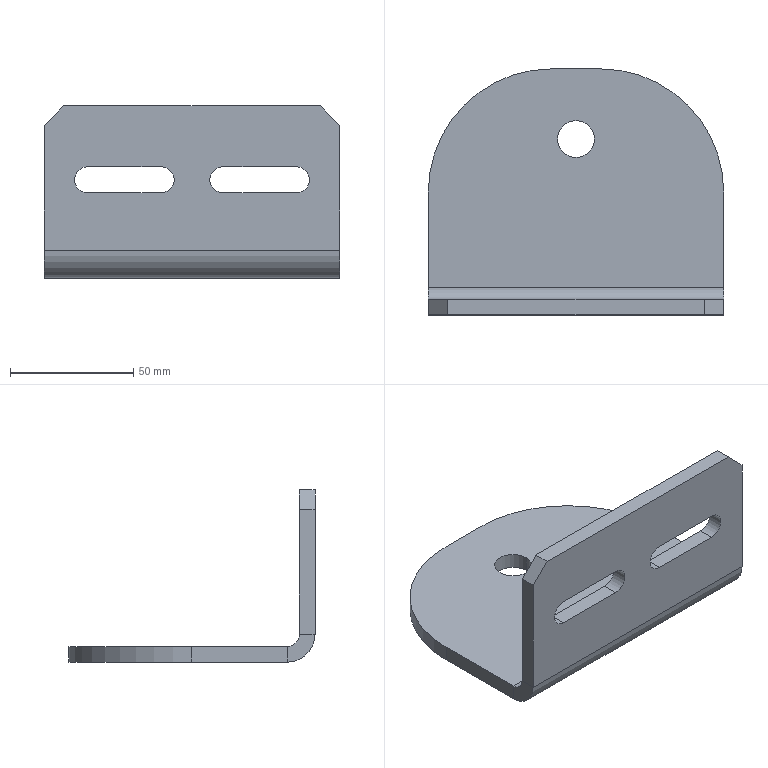Part | STEP file | BASE POLEA_B_SHEET METAL | 1 solid | 28 faces | box 120 x 100 x 70 mm | volume 108585 mm3 | plane 18 | cylinder 10 | commonest cylinder face diameters 10.5 x4 15 x2 100 x2 10 x1 22.7 x1
STEP:
#1=CARTESIAN_POINT('',(-7.5,71.5,0.));
#2=VERTEX_POINT('',#1);
#3=CARTESIAN_POINT('',(7.5,71.5,0.));
#4=VERTEX_POINT('',#3);
#5=CARTESIAN_POINT('',(0.,71.5,0.));
#6=DIRECTION('',(0.,0.,1.));
#7=DIRECTION('',(1.,0.,0.));
#8=AXIS2_PLACEMENT_3D('',#5,#6,#7);
#9=CIRCLE('',#8,7.5);
#10=EDGE_CURVE('',#2,#4,#9,.T.);
#11=ORIENTED_EDGE('',*,*,#10,.F.);
#12=CARTESIAN_POINT('',(-7.5,71.5,6.35));
#13=VERTEX_POINT('',#12);
#14=CARTESIAN_POINT('',(-7.5,71.5,-3.65));
#15=DIRECTION('',(0.,0.,1.));
#16=VECTOR('',#15,1000.);
#17=LINE('',#14,#16);
#18=EDGE_CURVE('',#2,#13,#17,.T.);
#19=ORIENTED_EDGE('',*,*,#18,.T.);
#20=CARTESIAN_POINT('',(7.5,71.5,6.35));
#21=VERTEX_POINT('',#20);
#22=CARTESIAN_POINT('',(0.,71.5,6.35));
#23=DIRECTION('',(0.,0.,1.));
#24=DIRECTION('',(1.,0.,0.));
#25=AXIS2_PLACEMENT_3D('',#22,#23,#24);
#26=CIRCLE('',#25,7.5);
#27=EDGE_CURVE('',#13,#21,#26,.T.);
#28=ORIENTED_EDGE('',*,*,#27,.T.);
#29=CARTESIAN_POINT('',(7.5,71.5,-3.65));
#30=DIRECTION('',(0.,0.,1.));
#31=VECTOR('',#30,1000.);
#32=LINE('',#29,#31);
#33=EDGE_CURVE('',#4,#21,#32,.T.);
#34=ORIENTED_EDGE('',*,*,#33,.F.);
#35=EDGE_LOOP('',(#11,#19,#28,#34));
#36=FACE_OUTER_BOUND('',#35,.T.);
#37=CARTESIAN_POINT('',(0.,71.5,-3.65));
#38=DIRECTION('',(0.,0.,1.));
#39=DIRECTION('',(1.,0.,0.));
#40=AXIS2_PLACEMENT_3D('',#37,#38,#39);
#41=CYLINDRICAL_SURFACE('',#40,7.5);
#42=ADVANCED_FACE('',(#36),#41,.F.);
#43=CARTESIAN_POINT('',(60.,0.,11.35));
#44=VERTEX_POINT('',#43);
#45=CARTESIAN_POINT('',(60.,6.35,11.35));
#46=VERTEX_POINT('',#45);
#47=CARTESIAN_POINT('',(60.,0.,11.35));
#48=DIRECTION('',(0.,1.,0.));
#49=VECTOR('',#48,1000.);
#50=LINE('',#47,#49);
#51=EDGE_CURVE('',#44,#46,#50,.T.);
#52=ORIENTED_EDGE('',*,*,#51,.F.);
#53=CARTESIAN_POINT('',(60.,11.35,0.));
#54=VERTEX_POINT('',#53);
#55=CARTESIAN_POINT('',(60.,11.35,11.35));
#56=DIRECTION('',(1.,0.,0.));
#57=DIRECTION('',(0.,0.,1.));
#58=AXIS2_PLACEMENT_3D('',#55,#56,#57);
#59=CIRCLE('',#58,11.35);
#60=EDGE_CURVE('',#44,#54,#59,.T.);
#61=ORIENTED_EDGE('',*,*,#60,.T.);
#62=CARTESIAN_POINT('',(60.,11.35,6.35));
#63=VERTEX_POINT('',#62);
#64=CARTESIAN_POINT('',(60.,11.35,6.35));
#65=DIRECTION('',(0.,0.,-1.));
#66=VECTOR('',#65,1000.);
#67=LINE('',#64,#66);
#68=EDGE_CURVE('',#63,#54,#67,.T.);
#69=ORIENTED_EDGE('',*,*,#68,.F.);
#70=CARTESIAN_POINT('',(60.,11.35,11.35));
#71=DIRECTION('',(1.,0.,0.));
#72=DIRECTION('',(0.,0.,-1.));
#73=AXIS2_PLACEMENT_3D('',#70,#71,#72);
#74=CIRCLE('',#73,5.);
#75=EDGE_CURVE('',#46,#63,#74,.T.);
#76=ORIENTED_EDGE('',*,*,#75,.F.);
#77=EDGE_LOOP('',(#52,#61,#69,#76));
#78=FACE_OUTER_BOUND('',#77,.T.);
#79=CARTESIAN_POINT('',(60.,0.,11.35));
#80=DIRECTION('',(1.,0.,0.));
#81=DIRECTION('',(0.,0.,-1.));
#82=AXIS2_PLACEMENT_3D('',#79,#80,#81);
#83=PLANE('',#82);
#84=ADVANCED_FACE('',(#78),#83,.T.);
#85=CARTESIAN_POINT('',(60.,6.35,62.));
#86=VERTEX_POINT('',#85);
#87=CARTESIAN_POINT('',(60.,6.35,70.));
#88=DIRECTION('',(0.,0.,-1.));
#89=VECTOR('',#88,1000.);
#90=LINE('',#87,#89);
#91=EDGE_CURVE('',#86,#46,#90,.T.);
#92=ORIENTED_EDGE('',*,*,#91,.F.);
#93=CARTESIAN_POINT('',(60.,0.,62.));
#94=VERTEX_POINT('',#93);
#95=CARTESIAN_POINT('',(60.,11.35,62.));
#96=DIRECTION('',(0.,-1.,0.));
#97=VECTOR('',#96,1000.);
#98=LINE('',#95,#97);
#99=EDGE_CURVE('',#86,#94,#98,.T.);
#100=ORIENTED_EDGE('',*,*,#99,.T.);
#101=CARTESIAN_POINT('',(60.,0.,70.));
#102=DIRECTION('',(0.,0.,-1.));
#103=VECTOR('',#102,1000.);
#104=LINE('',#101,#103);
#105=EDGE_CURVE('',#94,#44,#104,.T.);
#106=ORIENTED_EDGE('',*,*,#105,.T.);
#107=ORIENTED_EDGE('',*,*,#51,.T.);
#108=EDGE_LOOP('',(#92,#100,#106,#107));
#109=FACE_OUTER_BOUND('',#108,.T.);
#110=CARTESIAN_POINT('',(60.,11.35,6.35));
#111=DIRECTION('',(1.,0.,0.));
#112=DIRECTION('',(0.,0.,-1.));
#113=AXIS2_PLACEMENT_3D('',#110,#111,#112);
#114=PLANE('',#113);
#115=ADVANCED_FACE('',(#109),#114,.T.);
#116=CARTESIAN_POINT('',(-60.,11.35,0.));
#117=VERTEX_POINT('',#116);
#118=CARTESIAN_POINT('',(-60.,11.35,6.35));
#119=VERTEX_POINT('',#118);
#120=CARTESIAN_POINT('',(-60.,11.35,0.));
#121=DIRECTION('',(0.,0.,1.));
#122=VECTOR('',#121,1000.);
#123=LINE('',#120,#122);
#124=EDGE_CURVE('',#117,#119,#123,.T.);
#125=ORIENTED_EDGE('',*,*,#124,.F.);
#126=CARTESIAN_POINT('',(-60.,0.,11.35));
#127=VERTEX_POINT('',#126);
#128=CARTESIAN_POINT('',(-60.,11.35,11.35));
#129=DIRECTION('',(1.,0.,0.));
#130=DIRECTION('',(0.,0.,1.));
#131=AXIS2_PLACEMENT_3D('',#128,#129,#130);
#132=CIRCLE('',#131,11.35);
#133=EDGE_CURVE('',#127,#117,#132,.T.);
#134=ORIENTED_EDGE('',*,*,#133,.F.);
#135=CARTESIAN_POINT('',(-60.,6.35,11.35));
#136=VERTEX_POINT('',#135);
#137=CARTESIAN_POINT('',(-60.,6.35,11.35));
#138=DIRECTION('',(0.,-1.,0.));
#139=VECTOR('',#138,1000.);
#140=LINE('',#137,#139);
#141=EDGE_CURVE('',#136,#127,#140,.T.);
#142=ORIENTED_EDGE('',*,*,#141,.F.);
#143=CARTESIAN_POINT('',(-60.,11.35,11.35));
#144=DIRECTION('',(1.,0.,0.));
#145=DIRECTION('',(0.,0.,-1.));
#146=AXIS2_PLACEMENT_3D('',#143,#144,#145);
#147=CIRCLE('',#146,5.);
#148=EDGE_CURVE('',#136,#119,#147,.T.);
#149=ORIENTED_EDGE('',*,*,#148,.T.);
#150=EDGE_LOOP('',(#125,#134,#142,#149));
#151=FACE_OUTER_BOUND('',#150,.T.);
#152=CARTESIAN_POINT('',(-60.,11.35,0.));
#153=DIRECTION('',(-1.,0.,0.));
#154=DIRECTION('',(0.,0.,1.));
#155=AXIS2_PLACEMENT_3D('',#152,#153,#154);
#156=PLANE('',#155);
#157=ADVANCED_FACE('',(#151),#156,.T.);
#158=CARTESIAN_POINT('',(-60.,50.,6.35));
#159=VERTEX_POINT('',#158);
#160=CARTESIAN_POINT('',(-60.,0.,6.35));
#161=DIRECTION('',(0.,1.,0.));
#162=VECTOR('',#161,1000.);
#163=LINE('',#160,#162);
#164=EDGE_CURVE('',#119,#159,#163,.T.);
#165=ORIENTED_EDGE('',*,*,#164,.T.);
#166=CARTESIAN_POINT('',(-60.,50.,0.));
#167=VERTEX_POINT('',#166);
#168=CARTESIAN_POINT('',(-60.,50.,11.35));
#169=DIRECTION('',(0.,0.,-1.));
#170=VECTOR('',#169,1000.);
#171=LINE('',#168,#170);
#172=EDGE_CURVE('',#159,#167,#171,.T.);
#173=ORIENTED_EDGE('',*,*,#172,.T.);
#174=CARTESIAN_POINT('',(-60.,0.,0.));
#175=DIRECTION('',(0.,1.,0.));
#176=VECTOR('',#175,1000.);
#177=LINE('',#174,#176);
#178=EDGE_CURVE('',#117,#167,#177,.T.);
#179=ORIENTED_EDGE('',*,*,#178,.F.);
#180=ORIENTED_EDGE('',*,*,#124,.T.);
#181=EDGE_LOOP('',(#165,#173,#179,#180));
#182=FACE_OUTER_BOUND('',#181,.T.);
#183=CARTESIAN_POINT('',(-60.,6.35,11.35));
#184=DIRECTION('',(-1.,0.,0.));
#185=DIRECTION('',(0.,0.,1.));
#186=AXIS2_PLACEMENT_3D('',#183,#184,#185);
#187=PLANE('',#186);
#188=ADVANCED_FACE('',(#182),#187,.T.);
#189=CARTESIAN_POINT('',(0.,71.5,0.));
#190=DIRECTION('',(0.,0.,1.));
#191=DIRECTION('',(1.,0.,0.));
#192=AXIS2_PLACEMENT_3D('',#189,#190,#191);
#193=CIRCLE('',#192,7.5);
#194=EDGE_CURVE('',#4,#2,#193,.T.);
#195=ORIENTED_EDGE('',*,*,#194,.T.);
#196=ORIENTED_EDGE('',*,*,#10,.T.);
#197=EDGE_LOOP('',(#195,#196));
#198=FACE_BOUND('',#197,.T.);
#199=ORIENTED_EDGE('',*,*,#178,.T.);
#200=CARTESIAN_POINT('',(-10.,100.,0.));
#201=VERTEX_POINT('',#200);
#202=CARTESIAN_POINT('',(-10.,50.,0.));
#203=DIRECTION('',(0.,0.,-1.));
#204=DIRECTION('',(1.,0.,0.));
#205=AXIS2_PLACEMENT_3D('',#202,#203,#204);
#206=CIRCLE('',#205,50.);
#207=EDGE_CURVE('',#167,#201,#206,.T.);
#208=ORIENTED_EDGE('',*,*,#207,.T.);
#209=CARTESIAN_POINT('',(10.,100.,0.));
#210=VERTEX_POINT('',#209);
#211=CARTESIAN_POINT('',(60.,100.,0.));
#212=DIRECTION('',(-1.,0.,0.));
#213=VECTOR('',#212,1000.);
#214=LINE('',#211,#213);
#215=EDGE_CURVE('',#210,#201,#214,.T.);
#216=ORIENTED_EDGE('',*,*,#215,.F.);
#217=CARTESIAN_POINT('',(60.,50.,0.));
#218=VERTEX_POINT('',#217);
#219=CARTESIAN_POINT('',(10.,50.,0.));
#220=DIRECTION('',(0.,0.,-1.));
#221=DIRECTION('',(1.,0.,0.));
#222=AXIS2_PLACEMENT_3D('',#219,#220,#221);
#223=CIRCLE('',#222,50.);
#224=EDGE_CURVE('',#210,#218,#223,.T.);
#225=ORIENTED_EDGE('',*,*,#224,.T.);
#226=CARTESIAN_POINT('',(60.,0.,0.));
#227=DIRECTION('',(0.,1.,0.));
#228=VECTOR('',#227,1000.);
#229=LINE('',#226,#228);
#230=EDGE_CURVE('',#54,#218,#229,.T.);
#231=ORIENTED_EDGE('',*,*,#230,.F.);
#232=CARTESIAN_POINT('',(60.,11.35,0.));
#233=DIRECTION('',(-1.,0.,0.));
#234=VECTOR('',#233,1000.);
#235=LINE('',#232,#234);
#236=EDGE_CURVE('',#54,#117,#235,.T.);
#237=ORIENTED_EDGE('',*,*,#236,.T.);
#238=EDGE_LOOP('',(#199,#208,#216,#225,#231,#237));
#239=FACE_OUTER_BOUND('',#238,.T.);
#240=CARTESIAN_POINT('',(60.,0.,0.));
#241=DIRECTION('',(0.,0.,1.));
#242=DIRECTION('',(1.,0.,0.));
#243=AXIS2_PLACEMENT_3D('',#240,#241,#242);
#244=PLANE('',#243);
#245=ADVANCED_FACE('',(#198,#239),#244,.F.);
#246=ORIENTED_EDGE('',*,*,#215,.T.);
#247=CARTESIAN_POINT('',(-10.,100.,6.35));
#248=VERTEX_POINT('',#247);
#249=CARTESIAN_POINT('',(-10.,100.,6.35));
#250=DIRECTION('',(0.,0.,1.));
#251=VECTOR('',#250,1000.);
#252=LINE('',#249,#251);
#253=EDGE_CURVE('',#201,#248,#252,.T.);
#254=ORIENTED_EDGE('',*,*,#253,.T.);
#255=CARTESIAN_POINT('',(10.,100.,6.35));
#256=VERTEX_POINT('',#255);
#257=CARTESIAN_POINT('',(60.,100.,6.35));
#258=DIRECTION('',(-1.,0.,0.));
#259=VECTOR('',#258,1000.);
#260=LINE('',#257,#259);
#261=EDGE_CURVE('',#256,#248,#260,.T.);
#262=ORIENTED_EDGE('',*,*,#261,.F.);
#263=CARTESIAN_POINT('',(10.,100.,6.35));
#264=DIRECTION('',(0.,0.,-1.));
#265=VECTOR('',#264,1000.);
#266=LINE('',#263,#265);
#267=EDGE_CURVE('',#256,#210,#266,.T.);
#268=ORIENTED_EDGE('',*,*,#267,.T.);
#269=EDGE_LOOP('',(#246,#254,#262,#268));
#270=FACE_OUTER_BOUND('',#269,.T.);
#271=CARTESIAN_POINT('',(60.,100.,6.35));
#272=DIRECTION('',(0.,1.,0.));
#273=DIRECTION('',(0.,0.,1.));
#274=AXIS2_PLACEMENT_3D('',#271,#272,#273);
#275=PLANE('',#274);
#276=ADVANCED_FACE('',(#270),#275,.T.);
#277=CARTESIAN_POINT('',(0.,71.5,6.35));
#278=DIRECTION('',(0.,0.,1.));
#279=DIRECTION('',(1.,0.,0.));
#280=AXIS2_PLACEMENT_3D('',#277,#278,#279);
#281=CIRCLE('',#280,7.5);
#282=EDGE_CURVE('',#21,#13,#281,.T.);
#283=ORIENTED_EDGE('',*,*,#282,.F.);
#284=ORIENTED_EDGE('',*,*,#27,.F.);
#285=EDGE_LOOP('',(#283,#284));
#286=FACE_BOUND('',#285,.T.);
#287=ORIENTED_EDGE('',*,*,#261,.T.);
#288=CARTESIAN_POINT('',(-10.,50.,6.35));
#289=DIRECTION('',(0.,0.,1.));
#290=DIRECTION('',(1.,0.,0.));
#291=AXIS2_PLACEMENT_3D('',#288,#289,#290);
#292=CIRCLE('',#291,50.);
#293=EDGE_CURVE('',#248,#159,#292,.T.);
#294=ORIENTED_EDGE('',*,*,#293,.T.);
#295=ORIENTED_EDGE('',*,*,#164,.F.);
#296=CARTESIAN_POINT('',(60.,11.35,6.35));
#297=DIRECTION('',(-1.,0.,0.));
#298=VECTOR('',#297,1000.);
#299=LINE('',#296,#298);
#300=EDGE_CURVE('',#63,#119,#299,.T.);
#301=ORIENTED_EDGE('',*,*,#300,.F.);
#302=CARTESIAN_POINT('',(60.,50.,6.35));
#303=VERTEX_POINT('',#302);
#304=CARTESIAN_POINT('',(60.,0.,6.35));
#305=DIRECTION('',(0.,1.,0.));
#306=VECTOR('',#305,1000.);
#307=LINE('',#304,#306);
#308=EDGE_CURVE('',#63,#303,#307,.T.);
#309=ORIENTED_EDGE('',*,*,#308,.T.);
#310=CARTESIAN_POINT('',(10.,50.,6.35));
#311=DIRECTION('',(0.,0.,1.));
#312=DIRECTION('',(1.,0.,0.));
#313=AXIS2_PLACEMENT_3D('',#310,#311,#312);
#314=CIRCLE('',#313,50.);
#315=EDGE_CURVE('',#303,#256,#314,.T.);
#316=ORIENTED_EDGE('',*,*,#315,.T.);
#317=EDGE_LOOP('',(#287,#294,#295,#301,#309,#316));
#318=FACE_OUTER_BOUND('',#317,.T.);
#319=CARTESIAN_POINT('',(60.,0.,6.35));
#320=DIRECTION('',(0.,0.,1.));
#321=DIRECTION('',(1.,0.,0.));
#322=AXIS2_PLACEMENT_3D('',#319,#320,#321);
#323=PLANE('',#322);
#324=ADVANCED_FACE('',(#286,#318),#323,.T.);
#325=ORIENTED_EDGE('',*,*,#148,.F.);
#326=CARTESIAN_POINT('',(60.,6.35,11.35));
#327=DIRECTION('',(-1.,0.,0.));
#328=VECTOR('',#327,1000.);
#329=LINE('',#326,#328);
#330=EDGE_CURVE('',#46,#136,#329,.T.);
#331=ORIENTED_EDGE('',*,*,#330,.F.);
#332=ORIENTED_EDGE('',*,*,#75,.T.);
#333=ORIENTED_EDGE('',*,*,#300,.T.);
#334=EDGE_LOOP('',(#325,#331,#332,#333));
#335=FACE_OUTER_BOUND('',#334,.T.);
#336=CARTESIAN_POINT('',(60.,11.35,11.35));
#337=DIRECTION('',(-1.,0.,0.));
#338=DIRECTION('',(0.,0.,1.));
#339=AXIS2_PLACEMENT_3D('',#336,#337,#338);
#340=CYLINDRICAL_SURFACE('',#339,5.);
#341=ADVANCED_FACE('',(#335),#340,.F.);
#342=CARTESIAN_POINT('',(-42.5,6.35,34.75));
#343=VERTEX_POINT('',#342);
#344=CARTESIAN_POINT('',(-42.5,6.35,45.25));
#345=VERTEX_POINT('',#344);
#346=CARTESIAN_POINT('',(-42.5,6.35,40.));
#347=DIRECTION('',(0.,1.,0.));
#348=DIRECTION('',(0.,0.,1.));
#349=AXIS2_PLACEMENT_3D('',#346,#347,#348);
#350=CIRCLE('',#349,5.25);
#351=EDGE_CURVE('',#343,#345,#350,.T.);
#352=ORIENTED_EDGE('',*,*,#351,.F.);
#353=CARTESIAN_POINT('',(-12.5,6.35,34.75));
#354=VERTEX_POINT('',#353);
#355=CARTESIAN_POINT('',(-42.5,6.35,34.75));
#356=DIRECTION('',(-1.,0.,0.));
#357=VECTOR('',#356,1000.);
#358=LINE('',#355,#357);
#359=EDGE_CURVE('',#354,#343,#358,.T.);
#360=ORIENTED_EDGE('',*,*,#359,.F.);
#361=CARTESIAN_POINT('',(-12.5,6.35,45.25));
#362=VERTEX_POINT('',#361);
#363=CARTESIAN_POINT('',(-12.5,6.35,40.));
#364=DIRECTION('',(0.,1.,0.));
#365=DIRECTION('',(0.,0.,1.));
#366=AXIS2_PLACEMENT_3D('',#363,#364,#365);
#367=CIRCLE('',#366,5.25);
#368=EDGE_CURVE('',#362,#354,#367,.T.);
#369=ORIENTED_EDGE('',*,*,#368,.F.);
#370=CARTESIAN_POINT('',(-42.5,6.35,45.25));
#371=DIRECTION('',(1.,0.,0.));
#372=VECTOR('',#371,1000.);
#373=LINE('',#370,#372);
#374=EDGE_CURVE('',#345,#362,#373,.T.);
#375=ORIENTED_EDGE('',*,*,#374,.F.);
#376=EDGE_LOOP('',(#352,#360,#369,#375));
#377=FACE_BOUND('',#376,.T.);
#378=CARTESIAN_POINT('',(42.5,6.35,45.25));
#379=VERTEX_POINT('',#378);
#380=CARTESIAN_POINT('',(42.5,6.35,34.75));
#381=VERTEX_POINT('',#380);
#382=CARTESIAN_POINT('',(42.5,6.35,40.));
#383=DIRECTION('',(0.,1.,0.));
#384=DIRECTION('',(0.,0.,-1.));
#385=AXIS2_PLACEMENT_3D('',#382,#383,#384);
#386=CIRCLE('',#385,5.25);
#387=EDGE_CURVE('',#379,#381,#386,.T.);
#388=ORIENTED_EDGE('',*,*,#387,.F.);
#389=CARTESIAN_POINT('',(12.5,6.35,45.25));
#390=VERTEX_POINT('',#389);
#391=CARTESIAN_POINT('',(42.5,6.35,45.25));
#392=DIRECTION('',(1.,0.,0.));
#393=VECTOR('',#392,1000.);
#394=LINE('',#391,#393);
#395=EDGE_CURVE('',#390,#379,#394,.T.);
#396=ORIENTED_EDGE('',*,*,#395,.F.);
#397=CARTESIAN_POINT('',(12.5,6.35,34.75));
#398=VERTEX_POINT('',#397);
#399=CARTESIAN_POINT('',(12.5,6.35,40.));
#400=DIRECTION('',(0.,1.,0.));
#401=DIRECTION('',(0.,0.,-1.));
#402=AXIS2_PLACEMENT_3D('',#399,#400,#401);
#403=CIRCLE('',#402,5.25);
#404=EDGE_CURVE('',#398,#390,#403,.T.);
#405=ORIENTED_EDGE('',*,*,#404,.F.);
#406=CARTESIAN_POINT('',(42.5,6.35,34.75));
#407=DIRECTION('',(-1.,0.,0.));
#408=VECTOR('',#407,1000.);
#409=LINE('',#406,#408);
#410=EDGE_CURVE('',#381,#398,#409,.T.);
#411=ORIENTED_EDGE('',*,*,#410,.F.);
#412=EDGE_LOOP('',(#388,#396,#405,#411));
#413=FACE_BOUND('',#412,.T.);
#414=CARTESIAN_POINT('',(-60.,6.35,62.));
#415=VERTEX_POINT('',#414);
#416=CARTESIAN_POINT('',(-60.,6.35,70.));
#417=DIRECTION('',(0.,0.,-1.));
#418=VECTOR('',#417,1000.);
#419=LINE('',#416,#418);
#420=EDGE_CURVE('',#415,#136,#419,.T.);
#421=ORIENTED_EDGE('',*,*,#420,.F.);
#422=CARTESIAN_POINT('',(-52.,6.35,70.));
#423=VERTEX_POINT('',#422);
#424=CARTESIAN_POINT('',(4.,6.35,126.));
#425=DIRECTION('',(0.7071,0.,0.7071));
#426=VECTOR('',#425,1000.);
#427=LINE('',#424,#426);
#428=EDGE_CURVE('',#415,#423,#427,.T.);
#429=ORIENTED_EDGE('',*,*,#428,.T.);
#430=CARTESIAN_POINT('',(52.,6.35,70.));
#431=VERTEX_POINT('',#430);
#432=CARTESIAN_POINT('',(60.,6.35,70.));
#433=DIRECTION('',(-1.,0.,0.));
#434=VECTOR('',#433,1000.);
#435=LINE('',#432,#434);
#436=EDGE_CURVE('',#431,#423,#435,.T.);
#437=ORIENTED_EDGE('',*,*,#436,.F.);
#438=CARTESIAN_POINT('',(56.,6.35,66.));
#439=DIRECTION('',(0.7071,0.,-0.7071));
#440=VECTOR('',#439,1000.);
#441=LINE('',#438,#440);
#442=EDGE_CURVE('',#431,#86,#441,.T.);
#443=ORIENTED_EDGE('',*,*,#442,.T.);
#444=ORIENTED_EDGE('',*,*,#91,.T.);
#445=ORIENTED_EDGE('',*,*,#330,.T.);
#446=EDGE_LOOP('',(#421,#429,#437,#443,#444,#445));
#447=FACE_OUTER_BOUND('',#446,.T.);
#448=CARTESIAN_POINT('',(60.,6.35,70.));
#449=DIRECTION('',(0.,1.,0.));
#450=DIRECTION('',(0.,0.,1.));
#451=AXIS2_PLACEMENT_3D('',#448,#449,#450);
#452=PLANE('',#451);
#453=ADVANCED_FACE('',(#377,#413,#447),#452,.T.);
#454=ORIENTED_EDGE('',*,*,#436,.T.);
#455=CARTESIAN_POINT('',(-52.,0.,70.));
#456=VERTEX_POINT('',#455);
#457=CARTESIAN_POINT('',(-52.,0.,70.));
#458=DIRECTION('',(0.,-1.,0.));
#459=VECTOR('',#458,1000.);
#460=LINE('',#457,#459);
#461=EDGE_CURVE('',#423,#456,#460,.T.);
#462=ORIENTED_EDGE('',*,*,#461,.T.);
#463=CARTESIAN_POINT('',(52.,0.,70.));
#464=VERTEX_POINT('',#463);
#465=CARTESIAN_POINT('',(60.,0.,70.));
#466=DIRECTION('',(-1.,0.,0.));
#467=VECTOR('',#466,1000.);
#468=LINE('',#465,#467);
#469=EDGE_CURVE('',#464,#456,#468,.T.);
#470=ORIENTED_EDGE('',*,*,#469,.F.);
#471=CARTESIAN_POINT('',(52.,0.,70.));
#472=DIRECTION('',(0.,1.,0.));
#473=VECTOR('',#472,1000.);
#474=LINE('',#471,#473);
#475=EDGE_CURVE('',#464,#431,#474,.T.);
#476=ORIENTED_EDGE('',*,*,#475,.T.);
#477=EDGE_LOOP('',(#454,#462,#470,#476));
#478=FACE_OUTER_BOUND('',#477,.T.);
#479=CARTESIAN_POINT('',(60.,0.,70.));
#480=DIRECTION('',(0.,0.,1.));
#481=DIRECTION('',(1.,0.,0.));
#482=AXIS2_PLACEMENT_3D('',#479,#480,#481);
#483=PLANE('',#482);
#484=ADVANCED_FACE('',(#478),#483,.T.);
#485=CARTESIAN_POINT('',(-12.5,0.,34.75));
#486=VERTEX_POINT('',#485);
#487=CARTESIAN_POINT('',(-42.5,0.,34.75));
#488=VERTEX_POINT('',#487);
#489=CARTESIAN_POINT('',(-42.5,0.,34.75));
#490=DIRECTION('',(-1.,0.,0.));
#491=VECTOR('',#490,1000.);
#492=LINE('',#489,#491);
#493=EDGE_CURVE('',#486,#488,#492,.T.);
#494=ORIENTED_EDGE('',*,*,#493,.T.);
#495=CARTESIAN_POINT('',(-42.5,0.,45.25));
#496=VERTEX_POINT('',#495);
#497=CARTESIAN_POINT('',(-42.5,0.,40.));
#498=DIRECTION('',(0.,1.,0.));
#499=DIRECTION('',(0.,0.,1.));
#500=AXIS2_PLACEMENT_3D('',#497,#498,#499);
#501=CIRCLE('',#500,5.25);
#502=EDGE_CURVE('',#488,#496,#501,.T.);
#503=ORIENTED_EDGE('',*,*,#502,.T.);
#504=CARTESIAN_POINT('',(-12.5,0.,45.25));
#505=VERTEX_POINT('',#504);
#506=CARTESIAN_POINT('',(-42.5,0.,45.25));
#507=DIRECTION('',(1.,0.,0.));
#508=VECTOR('',#507,1000.);
#509=LINE('',#506,#508);
#510=EDGE_CURVE('',#496,#505,#509,.T.);
#511=ORIENTED_EDGE('',*,*,#510,.T.);
#512=CARTESIAN_POINT('',(-12.5,0.,40.));
#513=DIRECTION('',(0.,1.,0.));
#514=DIRECTION('',(0.,0.,1.));
#515=AXIS2_PLACEMENT_3D('',#512,#513,#514);
#516=CIRCLE('',#515,5.25);
#517=EDGE_CURVE('',#505,#486,#516,.T.);
#518=ORIENTED_EDGE('',*,*,#517,.T.);
#519=EDGE_LOOP('',(#494,#503,#511,#518));
#520=FACE_BOUND('',#519,.T.);
#521=CARTESIAN_POINT('',(12.5,0.,45.25));
#522=VERTEX_POINT('',#521);
#523=CARTESIAN_POINT('',(42.5,0.,45.25));
#524=VERTEX_POINT('',#523);
#525=CARTESIAN_POINT('',(42.5,0.,45.25));
#526=DIRECTION('',(1.,0.,0.));
#527=VECTOR('',#526,1000.);
#528=LINE('',#525,#527);
#529=EDGE_CURVE('',#522,#524,#528,.T.);
#530=ORIENTED_EDGE('',*,*,#529,.T.);
#531=CARTESIAN_POINT('',(42.5,0.,34.75));
#532=VERTEX_POINT('',#531);
#533=CARTESIAN_POINT('',(42.5,0.,40.));
#534=DIRECTION('',(0.,1.,0.));
#535=DIRECTION('',(0.,0.,-1.));
#536=AXIS2_PLACEMENT_3D('',#533,#534,#535);
#537=CIRCLE('',#536,5.25);
#538=EDGE_CURVE('',#524,#532,#537,.T.);
#539=ORIENTED_EDGE('',*,*,#538,.T.);
#540=CARTESIAN_POINT('',(12.5,0.,34.75));
#541=VERTEX_POINT('',#540);
#542=CARTESIAN_POINT('',(42.5,0.,34.75));
#543=DIRECTION('',(-1.,0.,0.));
#544=VECTOR('',#543,1000.);
#545=LINE('',#542,#544);
#546=EDGE_CURVE('',#532,#541,#545,.T.);
#547=ORIENTED_EDGE('',*,*,#546,.T.);
#548=CARTESIAN_POINT('',(12.5,0.,40.));
#549=DIRECTION('',(0.,1.,0.));
#550=DIRECTION('',(0.,0.,-1.));
#551=AXIS2_PLACEMENT_3D('',#548,#549,#550);
#552=CIRCLE('',#551,5.25);
#553=EDGE_CURVE('',#541,#522,#552,.T.);
#554=ORIENTED_EDGE('',*,*,#553,.T.);
#555=EDGE_LOOP('',(#530,#539,#547,#554));
#556=FACE_BOUND('',#555,.T.);
#557=ORIENTED_EDGE('',*,*,#469,.T.);
#558=CARTESIAN_POINT('',(-60.,0.,62.));
#559=VERTEX_POINT('',#558);
#560=CARTESIAN_POINT('',(-60.,0.,62.));
#561=DIRECTION('',(-0.7071,0.,-0.7071));
#562=VECTOR('',#561,1000.);
#563=LINE('',#560,#562);
#564=EDGE_CURVE('',#456,#559,#563,.T.);
#565=ORIENTED_EDGE('',*,*,#564,.T.);
#566=CARTESIAN_POINT('',(-60.,0.,70.));
#567=DIRECTION('',(0.,0.,-1.));
#568=VECTOR('',#567,1000.);
#569=LINE('',#566,#568);
#570=EDGE_CURVE('',#559,#127,#569,.T.);
#571=ORIENTED_EDGE('',*,*,#570,.T.);
#572=CARTESIAN_POINT('',(60.,0.,11.35));
#573=DIRECTION('',(-1.,0.,0.));
#574=VECTOR('',#573,1000.);
#575=LINE('',#572,#574);
#576=EDGE_CURVE('',#44,#127,#575,.T.);
#577=ORIENTED_EDGE('',*,*,#576,.F.);
#578=ORIENTED_EDGE('',*,*,#105,.F.);
#579=CARTESIAN_POINT('',(52.,0.,70.));
#580=DIRECTION('',(-0.7071,0.,0.7071));
#581=VECTOR('',#580,1000.);
#582=LINE('',#579,#581);
#583=EDGE_CURVE('',#94,#464,#582,.T.);
#584=ORIENTED_EDGE('',*,*,#583,.T.);
#585=EDGE_LOOP('',(#557,#565,#571,#577,#578,#584));
#586=FACE_OUTER_BOUND('',#585,.T.);
#587=CARTESIAN_POINT('',(60.,0.,70.));
#588=DIRECTION('',(0.,1.,0.));
#589=DIRECTION('',(0.,0.,1.));
#590=AXIS2_PLACEMENT_3D('',#587,#588,#589);
#591=PLANE('',#590);
#592=ADVANCED_FACE('',(#520,#556,#586),#591,.F.);
#593=ORIENTED_EDGE('',*,*,#133,.T.);
#594=ORIENTED_EDGE('',*,*,#236,.F.);
#595=ORIENTED_EDGE('',*,*,#60,.F.);
#596=ORIENTED_EDGE('',*,*,#576,.T.);
#597=EDGE_LOOP('',(#593,#594,#595,#596));
#598=FACE_OUTER_BOUND('',#597,.T.);
#599=CARTESIAN_POINT('',(60.,11.35,11.35));
#600=DIRECTION('',(-1.,0.,0.));
#601=DIRECTION('',(0.,0.,1.));
#602=AXIS2_PLACEMENT_3D('',#599,#600,#601);
#603=CYLINDRICAL_SURFACE('',#602,11.35);
#604=ADVANCED_FACE('',(#598),#603,.T.);
#605=ORIENTED_EDGE('',*,*,#230,.T.);
#606=CARTESIAN_POINT('',(60.,50.,11.35));
#607=DIRECTION('',(0.,0.,1.));
#608=VECTOR('',#607,1000.);
#609=LINE('',#606,#608);
#610=EDGE_CURVE('',#218,#303,#609,.T.);
#611=ORIENTED_EDGE('',*,*,#610,.T.);
#612=ORIENTED_EDGE('',*,*,#308,.F.);
#613=ORIENTED_EDGE('',*,*,#68,.T.);
#614=EDGE_LOOP('',(#605,#611,#612,#613));
#615=FACE_OUTER_BOUND('',#614,.T.);
#616=CARTESIAN_POINT('',(60.,11.35,11.35));
#617=DIRECTION('',(1.,0.,0.));
#618=DIRECTION('',(0.,0.,-1.));
#619=AXIS2_PLACEMENT_3D('',#616,#617,#618);
#620=PLANE('',#619);
#621=ADVANCED_FACE('',(#615),#620,.T.);
#622=ORIENTED_EDGE('',*,*,#570,.F.);
#623=CARTESIAN_POINT('',(-60.,6.35,62.));
#624=DIRECTION('',(0.,1.,0.));
#625=VECTOR('',#624,1000.);
#626=LINE('',#623,#625);
#627=EDGE_CURVE('',#559,#415,#626,.T.);
#628=ORIENTED_EDGE('',*,*,#627,.T.);
#629=ORIENTED_EDGE('',*,*,#420,.T.);
#630=ORIENTED_EDGE('',*,*,#141,.T.);
#631=EDGE_LOOP('',(#622,#628,#629,#630));
#632=FACE_OUTER_BOUND('',#631,.T.);
#633=CARTESIAN_POINT('',(-60.,11.35,11.35));
#634=DIRECTION('',(1.,0.,0.));
#635=DIRECTION('',(0.,0.,-1.));
#636=AXIS2_PLACEMENT_3D('',#633,#634,#635);
#637=PLANE('',#636);
#638=ADVANCED_FACE('',(#632),#637,.F.);
#639=ORIENTED_EDGE('',*,*,#18,.F.);
#640=ORIENTED_EDGE('',*,*,#194,.F.);
#641=ORIENTED_EDGE('',*,*,#33,.T.);
#642=ORIENTED_EDGE('',*,*,#282,.T.);
#643=EDGE_LOOP('',(#639,#640,#641,#642));
#644=FACE_OUTER_BOUND('',#643,.T.);
#645=CARTESIAN_POINT('',(0.,71.5,-3.65));
#646=DIRECTION('',(0.,0.,1.));
#647=DIRECTION('',(1.,0.,0.));
#648=AXIS2_PLACEMENT_3D('',#645,#646,#647);
#649=CYLINDRICAL_SURFACE('',#648,7.5);
#650=ADVANCED_FACE('',(#644),#649,.F.);
#651=ORIENTED_EDGE('',*,*,#293,.F.);
#652=ORIENTED_EDGE('',*,*,#253,.F.);
#653=ORIENTED_EDGE('',*,*,#207,.F.);
#654=ORIENTED_EDGE('',*,*,#172,.F.);
#655=EDGE_LOOP('',(#651,#652,#653,#654));
#656=FACE_OUTER_BOUND('',#655,.T.);
#657=CARTESIAN_POINT('',(-10.,50.,11.35));
#658=DIRECTION('',(0.,0.,-1.));
#659=DIRECTION('',(-1.,0.,0.));
#660=AXIS2_PLACEMENT_3D('',#657,#658,#659);
#661=CYLINDRICAL_SURFACE('',#660,50.);
#662=ADVANCED_FACE('',(#656),#661,.T.);
#663=ORIENTED_EDGE('',*,*,#315,.F.);
#664=ORIENTED_EDGE('',*,*,#610,.F.);
#665=ORIENTED_EDGE('',*,*,#224,.F.);
#666=ORIENTED_EDGE('',*,*,#267,.F.);
#667=EDGE_LOOP('',(#663,#664,#665,#666));
#668=FACE_OUTER_BOUND('',#667,.T.);
#669=CARTESIAN_POINT('',(10.,50.,6.35));
#670=DIRECTION('',(0.,0.,-1.));
#671=DIRECTION('',(-1.,0.,0.));
#672=AXIS2_PLACEMENT_3D('',#669,#670,#671);
#673=CYLINDRICAL_SURFACE('',#672,50.);
#674=ADVANCED_FACE('',(#668),#673,.T.);
#675=ORIENTED_EDGE('',*,*,#564,.F.);
#676=ORIENTED_EDGE('',*,*,#461,.F.);
#677=ORIENTED_EDGE('',*,*,#428,.F.);
#678=ORIENTED_EDGE('',*,*,#627,.F.);
#679=EDGE_LOOP('',(#675,#676,#677,#678));
#680=FACE_OUTER_BOUND('',#679,.T.);
#681=CARTESIAN_POINT('',(-60.,11.35,62.));
#682=DIRECTION('',(-0.7071,0.,0.7071));
#683=DIRECTION('',(0.,-1.,0.));
#684=AXIS2_PLACEMENT_3D('',#681,#682,#683);
#685=PLANE('',#684);
#686=ADVANCED_FACE('',(#680),#685,.T.);
#687=ORIENTED_EDGE('',*,*,#583,.F.);
#688=ORIENTED_EDGE('',*,*,#99,.F.);
#689=ORIENTED_EDGE('',*,*,#442,.F.);
#690=ORIENTED_EDGE('',*,*,#475,.F.);
#691=EDGE_LOOP('',(#687,#688,#689,#690));
#692=FACE_OUTER_BOUND('',#691,.T.);
#693=CARTESIAN_POINT('',(52.,0.,70.));
#694=DIRECTION('',(-0.7071,0.,-0.7071));
#695=DIRECTION('',(0.,1.,0.));
#696=AXIS2_PLACEMENT_3D('',#693,#694,#695);
#697=PLANE('',#696);
#698=ADVANCED_FACE('',(#692),#697,.F.);
#699=ORIENTED_EDGE('',*,*,#387,.T.);
#700=CARTESIAN_POINT('',(42.5,0.,34.75));
#701=DIRECTION('',(0.,1.,0.));
#702=VECTOR('',#701,1000.);
#703=LINE('',#700,#702);
#704=EDGE_CURVE('',#532,#381,#703,.T.);
#705=ORIENTED_EDGE('',*,*,#704,.F.);
#706=ORIENTED_EDGE('',*,*,#538,.F.);
#707=CARTESIAN_POINT('',(42.5,0.,45.25));
#708=DIRECTION('',(0.,1.,0.));
#709=VECTOR('',#708,1000.);
#710=LINE('',#707,#709);
#711=EDGE_CURVE('',#524,#379,#710,.T.);
#712=ORIENTED_EDGE('',*,*,#711,.T.);
#713=EDGE_LOOP('',(#699,#705,#706,#712));
#714=FACE_OUTER_BOUND('',#713,.T.);
#715=CARTESIAN_POINT('',(42.5,0.,40.));
#716=DIRECTION('',(0.,1.,0.));
#717=DIRECTION('',(0.,0.,1.));
#718=AXIS2_PLACEMENT_3D('',#715,#716,#717);
#719=CYLINDRICAL_SURFACE('',#718,5.25);
#720=ADVANCED_FACE('',(#714),#719,.F.);
#721=ORIENTED_EDGE('',*,*,#395,.T.);
#722=ORIENTED_EDGE('',*,*,#711,.F.);
#723=ORIENTED_EDGE('',*,*,#529,.F.);
#724=CARTESIAN_POINT('',(12.5,0.,45.25));
#725=DIRECTION('',(0.,1.,0.));
#726=VECTOR('',#725,1000.);
#727=LINE('',#724,#726);
#728=EDGE_CURVE('',#522,#390,#727,.T.);
#729=ORIENTED_EDGE('',*,*,#728,.T.);
#730=EDGE_LOOP('',(#721,#722,#723,#729));
#731=FACE_OUTER_BOUND('',#730,.T.);
#732=CARTESIAN_POINT('',(42.5,0.,45.25));
#733=DIRECTION('',(0.,0.,1.));
#734=DIRECTION('',(1.,0.,0.));
#735=AXIS2_PLACEMENT_3D('',#732,#733,#734);
#736=PLANE('',#735);
#737=ADVANCED_FACE('',(#731),#736,.F.);
#738=ORIENTED_EDGE('',*,*,#404,.T.);
#739=ORIENTED_EDGE('',*,*,#728,.F.);
#740=ORIENTED_EDGE('',*,*,#553,.F.);
#741=CARTESIAN_POINT('',(12.5,0.,34.75));
#742=DIRECTION('',(0.,1.,0.));
#743=VECTOR('',#742,1000.);
#744=LINE('',#741,#743);
#745=EDGE_CURVE('',#541,#398,#744,.T.);
#746=ORIENTED_EDGE('',*,*,#745,.T.);
#747=EDGE_LOOP('',(#738,#739,#740,#746));
#748=FACE_OUTER_BOUND('',#747,.T.);
#749=CARTESIAN_POINT('',(12.5,0.,40.));
#750=DIRECTION('',(0.,1.,0.));
#751=DIRECTION('',(0.,0.,1.));
#752=AXIS2_PLACEMENT_3D('',#749,#750,#751);
#753=CYLINDRICAL_SURFACE('',#752,5.25);
#754=ADVANCED_FACE('',(#748),#753,.F.);
#755=ORIENTED_EDGE('',*,*,#410,.T.);
#756=ORIENTED_EDGE('',*,*,#745,.F.);
#757=ORIENTED_EDGE('',*,*,#546,.F.);
#758=ORIENTED_EDGE('',*,*,#704,.T.);
#759=EDGE_LOOP('',(#755,#756,#757,#758));
#760=FACE_OUTER_BOUND('',#759,.T.);
#761=CARTESIAN_POINT('',(42.5,0.,34.75));
#762=DIRECTION('',(0.,0.,-1.));
#763=DIRECTION('',(-1.,0.,0.));
#764=AXIS2_PLACEMENT_3D('',#761,#762,#763);
#765=PLANE('',#764);
#766=ADVANCED_FACE('',(#760),#765,.F.);
#767=ORIENTED_EDGE('',*,*,#351,.T.);
#768=CARTESIAN_POINT('',(-42.5,0.,45.25));
#769=DIRECTION('',(0.,1.,0.));
#770=VECTOR('',#769,1000.);
#771=LINE('',#768,#770);
#772=EDGE_CURVE('',#496,#345,#771,.T.);
#773=ORIENTED_EDGE('',*,*,#772,.F.);
#774=ORIENTED_EDGE('',*,*,#502,.F.);
#775=CARTESIAN_POINT('',(-42.5,0.,34.75));
#776=DIRECTION('',(0.,1.,0.));
#777=VECTOR('',#776,1000.);
#778=LINE('',#775,#777);
#779=EDGE_CURVE('',#488,#343,#778,.T.);
#780=ORIENTED_EDGE('',*,*,#779,.T.);
#781=EDGE_LOOP('',(#767,#773,#774,#780));
#782=FACE_OUTER_BOUND('',#781,.T.);
#783=CARTESIAN_POINT('',(-42.5,0.,40.));
#784=DIRECTION('',(0.,1.,0.));
#785=DIRECTION('',(0.,0.,1.));
#786=AXIS2_PLACEMENT_3D('',#783,#784,#785);
#787=CYLINDRICAL_SURFACE('',#786,5.25);
#788=ADVANCED_FACE('',(#782),#787,.F.);
#789=ORIENTED_EDGE('',*,*,#359,.T.);
#790=ORIENTED_EDGE('',*,*,#779,.F.);
#791=ORIENTED_EDGE('',*,*,#493,.F.);
#792=CARTESIAN_POINT('',(-12.5,0.,34.75));
#793=DIRECTION('',(0.,1.,0.));
#794=VECTOR('',#793,1000.);
#795=LINE('',#792,#794);
#796=EDGE_CURVE('',#486,#354,#795,.T.);
#797=ORIENTED_EDGE('',*,*,#796,.T.);
#798=EDGE_LOOP('',(#789,#790,#791,#797));
#799=FACE_OUTER_BOUND('',#798,.T.);
#800=CARTESIAN_POINT('',(-42.5,0.,34.75));
#801=DIRECTION('',(0.,0.,-1.));
#802=DIRECTION('',(-1.,0.,0.));
#803=AXIS2_PLACEMENT_3D('',#800,#801,#802);
#804=PLANE('',#803);
#805=ADVANCED_FACE('',(#799),#804,.F.);
#806=ORIENTED_EDGE('',*,*,#368,.T.);
#807=ORIENTED_EDGE('',*,*,#796,.F.);
#808=ORIENTED_EDGE('',*,*,#517,.F.);
#809=CARTESIAN_POINT('',(-12.5,0.,45.25));
#810=DIRECTION('',(0.,1.,0.));
#811=VECTOR('',#810,1000.);
#812=LINE('',#809,#811);
#813=EDGE_CURVE('',#505,#362,#812,.T.);
#814=ORIENTED_EDGE('',*,*,#813,.T.);
#815=EDGE_LOOP('',(#806,#807,#808,#814));
#816=FACE_OUTER_BOUND('',#815,.T.);
#817=CARTESIAN_POINT('',(-12.5,0.,40.));
#818=DIRECTION('',(0.,1.,0.));
#819=DIRECTION('',(0.,0.,1.));
#820=AXIS2_PLACEMENT_3D('',#817,#818,#819);
#821=CYLINDRICAL_SURFACE('',#820,5.25);
#822=ADVANCED_FACE('',(#816),#821,.F.);
#823=ORIENTED_EDGE('',*,*,#374,.T.);
#824=ORIENTED_EDGE('',*,*,#813,.F.);
#825=ORIENTED_EDGE('',*,*,#510,.F.);
#826=ORIENTED_EDGE('',*,*,#772,.T.);
#827=EDGE_LOOP('',(#823,#824,#825,#826));
#828=FACE_OUTER_BOUND('',#827,.T.);
#829=CARTESIAN_POINT('',(-42.5,0.,45.25));
#830=DIRECTION('',(0.,0.,1.));
#831=DIRECTION('',(1.,0.,0.));
#832=AXIS2_PLACEMENT_3D('',#829,#830,#831);
#833=PLANE('',#832);
#834=ADVANCED_FACE('',(#828),#833,.F.);
#835=CLOSED_SHELL('',(#42,#84,#115,#157,#188,#245,#276,#324,#341,#453,#484,#592,#604,#621,#638,#650,#662,#674,#686,#698,#720,#737,#754,#766,#788,#805,#822,#834));
#836=MANIFOLD_SOLID_BREP('',#835);
#837=CARTESIAN_POINT('',(0.,0.,0.));
#838=DIRECTION('',(0.,0.,1.));
#839=DIRECTION('',(1.,0.,0.));
#840=AXIS2_PLACEMENT_3D('',#837,#838,#839);
#841=(LENGTH_UNIT()NAMED_UNIT(*)SI_UNIT(.MILLI.,.METRE.));
#842=UNCERTAINTY_MEASURE_WITH_UNIT(LENGTH_MEASURE(0.00001),#841,'','');
#843=(NAMED_UNIT(*)PLANE_ANGLE_UNIT()SI_UNIT($,.RADIAN.));
#844=(NAMED_UNIT(*)SI_UNIT($,.STERADIAN.)SOLID_ANGLE_UNIT());
#845=(GEOMETRIC_REPRESENTATION_CONTEXT(3)GLOBAL_UNCERTAINTY_ASSIGNED_CONTEXT((#842))GLOBAL_UNIT_ASSIGNED_CONTEXT((#841,#843,#844))REPRESENTATION_CONTEXT('',''));
#846=ADVANCED_BREP_SHAPE_REPRESENTATION('',(#836,#840),#845);